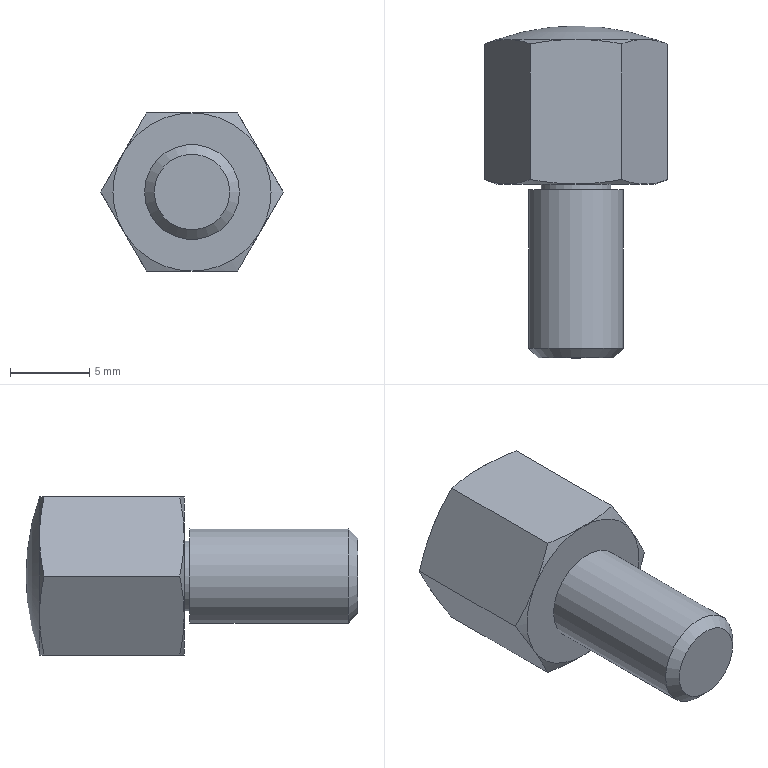Part | NX | features BREP 1 | 1 solid | 25 faces | box 11.547 x 21 x 10 mm | volume 1127 mm3 | cone 13 | plane 9 | cylinder 2 | sphere 1 | commonest cylinder face diameters 4.4 x1 6 x1
STEP:
#1=CARTESIAN_POINT('',(4.33,9.142,-2.5));
#2=VERTEX_POINT('',#1);
#3=CARTESIAN_POINT('',(4.33,9.142,2.5));
#4=VERTEX_POINT('',#3);
#5=CARTESIAN_POINT('',(0.,9.142,0.));
#6=DIRECTION('',(0.,-1.,0.));
#7=DIRECTION('',(1.,0.,0.));
#8=AXIS2_PLACEMENT_3D('',#5,#6,#7);
#9=CIRCLE('',#8,5.);
#10=EDGE_CURVE('',#2,#4,#9,.T.);
#11=ORIENTED_EDGE('',*,*,#10,.F.);
#12=CARTESIAN_POINT('',(0.,9.142,-5.));
#13=VERTEX_POINT('',#12);
#14=CARTESIAN_POINT('',(0.,9.142,0.));
#15=DIRECTION('',(0.,-1.,0.));
#16=DIRECTION('',(1.,0.,0.));
#17=AXIS2_PLACEMENT_3D('',#14,#15,#16);
#18=CIRCLE('',#17,5.);
#19=EDGE_CURVE('',#13,#2,#18,.T.);
#20=ORIENTED_EDGE('',*,*,#19,.F.);
#21=CARTESIAN_POINT('',(-4.33,9.142,-2.5));
#22=VERTEX_POINT('',#21);
#23=CARTESIAN_POINT('',(0.,9.142,0.));
#24=DIRECTION('',(0.,-1.,0.));
#25=DIRECTION('',(1.,0.,0.));
#26=AXIS2_PLACEMENT_3D('',#23,#24,#25);
#27=CIRCLE('',#26,5.);
#28=EDGE_CURVE('',#22,#13,#27,.T.);
#29=ORIENTED_EDGE('',*,*,#28,.F.);
#30=CARTESIAN_POINT('',(-4.33,9.142,2.5));
#31=VERTEX_POINT('',#30);
#32=CARTESIAN_POINT('',(0.,9.142,0.));
#33=DIRECTION('',(0.,-1.,0.));
#34=DIRECTION('',(1.,0.,0.));
#35=AXIS2_PLACEMENT_3D('',#32,#33,#34);
#36=CIRCLE('',#35,5.);
#37=EDGE_CURVE('',#31,#22,#36,.T.);
#38=ORIENTED_EDGE('',*,*,#37,.F.);
#39=CARTESIAN_POINT('',(0.,9.142,5.));
#40=VERTEX_POINT('',#39);
#41=CARTESIAN_POINT('',(0.,9.142,0.));
#42=DIRECTION('',(0.,-1.,0.));
#43=DIRECTION('',(1.,0.,0.));
#44=AXIS2_PLACEMENT_3D('',#41,#42,#43);
#45=CIRCLE('',#44,5.);
#46=EDGE_CURVE('',#40,#31,#45,.T.);
#47=ORIENTED_EDGE('',*,*,#46,.F.);
#48=CARTESIAN_POINT('',(0.,9.142,0.));
#49=DIRECTION('',(0.,-1.,0.));
#50=DIRECTION('',(1.,0.,0.));
#51=AXIS2_PLACEMENT_3D('',#48,#49,#50);
#52=CIRCLE('',#51,5.);
#53=EDGE_CURVE('',#4,#40,#52,.T.);
#54=ORIENTED_EDGE('',*,*,#53,.F.);
#55=EDGE_LOOP('',(#11,#20,#29,#38,#47,#54));
#56=FACE_BOUND('',#55,.T.);
#57=CARTESIAN_POINT('',(0.,-5.,0.));
#58=DIRECTION('',(0.,-1.,0.));
#59=DIRECTION('',(-1.,0.,0.));
#60=AXIS2_PLACEMENT_3D('',#57,#58,#59);
#61=SPHERICAL_SURFACE('',#60,15.);
#62=ADVANCED_FACE('',(#56),#61,.T.);
#63=CARTESIAN_POINT('',(2.2,0.,0.));
#64=VERTEX_POINT('',#63);
#65=CARTESIAN_POINT('',(0.,0.,0.));
#66=DIRECTION('',(0.,-1.,0.));
#67=DIRECTION('',(1.,0.,0.));
#68=AXIS2_PLACEMENT_3D('',#65,#66,#67);
#69=CIRCLE('',#68,2.2);
#70=EDGE_CURVE('',#64,#64,#69,.T.);
#71=ORIENTED_EDGE('',*,*,#70,.F.);
#72=EDGE_LOOP('',(#71));
#73=FACE_BOUND('',#72,.T.);
#74=CARTESIAN_POINT('',(4.33,0.,-2.5));
#75=VERTEX_POINT('',#74);
#76=CARTESIAN_POINT('',(4.33,0.,2.5));
#77=VERTEX_POINT('',#76);
#78=CARTESIAN_POINT('',(0.,0.,0.));
#79=DIRECTION('',(0.,-1.,0.));
#80=DIRECTION('',(1.,0.,0.));
#81=AXIS2_PLACEMENT_3D('',#78,#79,#80);
#82=CIRCLE('',#81,5.);
#83=EDGE_CURVE('',#75,#77,#82,.T.);
#84=ORIENTED_EDGE('',*,*,#83,.T.);
#85=CARTESIAN_POINT('',(0.,0.,5.));
#86=VERTEX_POINT('',#85);
#87=CARTESIAN_POINT('',(0.,0.,0.));
#88=DIRECTION('',(0.,-1.,0.));
#89=DIRECTION('',(1.,0.,0.));
#90=AXIS2_PLACEMENT_3D('',#87,#88,#89);
#91=CIRCLE('',#90,5.);
#92=EDGE_CURVE('',#77,#86,#91,.T.);
#93=ORIENTED_EDGE('',*,*,#92,.T.);
#94=CARTESIAN_POINT('',(-4.33,0.,2.5));
#95=VERTEX_POINT('',#94);
#96=CARTESIAN_POINT('',(0.,0.,0.));
#97=DIRECTION('',(0.,-1.,0.));
#98=DIRECTION('',(1.,0.,0.));
#99=AXIS2_PLACEMENT_3D('',#96,#97,#98);
#100=CIRCLE('',#99,5.);
#101=EDGE_CURVE('',#86,#95,#100,.T.);
#102=ORIENTED_EDGE('',*,*,#101,.T.);
#103=CARTESIAN_POINT('',(-4.33,0.,-2.5));
#104=VERTEX_POINT('',#103);
#105=CARTESIAN_POINT('',(0.,0.,0.));
#106=DIRECTION('',(0.,-1.,0.));
#107=DIRECTION('',(1.,0.,0.));
#108=AXIS2_PLACEMENT_3D('',#105,#106,#107);
#109=CIRCLE('',#108,5.);
#110=EDGE_CURVE('',#95,#104,#109,.T.);
#111=ORIENTED_EDGE('',*,*,#110,.T.);
#112=CARTESIAN_POINT('',(0.,0.,-5.));
#113=VERTEX_POINT('',#112);
#114=CARTESIAN_POINT('',(0.,0.,0.));
#115=DIRECTION('',(0.,-1.,0.));
#116=DIRECTION('',(1.,0.,0.));
#117=AXIS2_PLACEMENT_3D('',#114,#115,#116);
#118=CIRCLE('',#117,5.);
#119=EDGE_CURVE('',#104,#113,#118,.T.);
#120=ORIENTED_EDGE('',*,*,#119,.T.);
#121=CARTESIAN_POINT('',(0.,0.,0.));
#122=DIRECTION('',(0.,-1.,0.));
#123=DIRECTION('',(1.,0.,0.));
#124=AXIS2_PLACEMENT_3D('',#121,#122,#123);
#125=CIRCLE('',#124,5.);
#126=EDGE_CURVE('',#113,#75,#125,.T.);
#127=ORIENTED_EDGE('',*,*,#126,.T.);
#128=EDGE_LOOP('',(#84,#93,#102,#111,#120,#127));
#129=FACE_BOUND('',#128,.T.);
#130=CARTESIAN_POINT('',(3.6,0.,0.));
#131=DIRECTION('',(0.,-1.,0.));
#132=DIRECTION('',(0.,0.,-1.));
#133=AXIS2_PLACEMENT_3D('',#130,#131,#132);
#134=PLANE('',#133);
#135=ADVANCED_FACE('',(#73,#129),#134,.T.);
#136=CARTESIAN_POINT('',(2.2,-0.3667,0.));
#137=VERTEX_POINT('',#136);
#138=CARTESIAN_POINT('',(0.,-0.3667,0.));
#139=DIRECTION('',(0.,-1.,0.));
#140=DIRECTION('',(1.,0.,0.));
#141=AXIS2_PLACEMENT_3D('',#138,#139,#140);
#142=CIRCLE('',#141,2.2);
#143=EDGE_CURVE('',#137,#137,#142,.T.);
#144=ORIENTED_EDGE('',*,*,#143,.T.);
#145=EDGE_LOOP('',(#144));
#146=FACE_BOUND('',#145,.T.);
#147=CARTESIAN_POINT('',(3.,-0.3667,0.));
#148=VERTEX_POINT('',#147);
#149=CARTESIAN_POINT('',(0.,-0.3667,0.));
#150=DIRECTION('',(0.,-1.,0.));
#151=DIRECTION('',(1.,0.,0.));
#152=AXIS2_PLACEMENT_3D('',#149,#150,#151);
#153=CIRCLE('',#152,3.);
#154=EDGE_CURVE('',#148,#148,#153,.T.);
#155=ORIENTED_EDGE('',*,*,#154,.F.);
#156=EDGE_LOOP('',(#155));
#157=FACE_BOUND('',#156,.T.);
#158=CARTESIAN_POINT('',(2.6,-0.3667,0.));
#159=DIRECTION('',(0.,1.,0.));
#160=DIRECTION('',(-1.,0.,0.));
#161=AXIS2_PLACEMENT_3D('',#158,#159,#160);
#162=PLANE('',#161);
#163=ADVANCED_FACE('',(#146,#157),#162,.T.);
#164=CARTESIAN_POINT('',(2.386,-11.,0.));
#165=VERTEX_POINT('',#164);
#166=CARTESIAN_POINT('',(0.,-11.,0.));
#167=DIRECTION('',(0.,-1.,0.));
#168=DIRECTION('',(1.,0.,0.));
#169=AXIS2_PLACEMENT_3D('',#166,#167,#168);
#170=CIRCLE('',#169,2.386);
#171=EDGE_CURVE('',#165,#165,#170,.T.);
#172=ORIENTED_EDGE('',*,*,#171,.T.);
#173=EDGE_LOOP('',(#172));
#174=FACE_BOUND('',#173,.T.);
#175=CARTESIAN_POINT('',(1.193,-11.,0.));
#176=DIRECTION('',(0.,-1.,0.));
#177=DIRECTION('',(0.,0.,-1.));
#178=AXIS2_PLACEMENT_3D('',#175,#176,#177);
#179=PLANE('',#178);
#180=ADVANCED_FACE('',(#174),#179,.T.);
#181=CARTESIAN_POINT('',(-2.887,8.861,5.));
#182=VERTEX_POINT('',#181);
#183=CARTESIAN_POINT('',(0.,9.142,5.));
#184=CARTESIAN_POINT('',(-1.34,9.142,5.));
#185=CARTESIAN_POINT('',(-2.887,8.861,5.));
#186=(BOUNDED_CURVE()B_SPLINE_CURVE(2,(#183,#184,#185),.UNSPECIFIED.,.F.,.F.)B_SPLINE_CURVE_WITH_KNOTS((3,3),(0.,1.),.PIECEWISE_BEZIER_KNOTS.)CURVE()GEOMETRIC_REPRESENTATION_ITEM()RATIONAL_B_SPLINE_CURVE((1.,1.136,1.199))REPRESENTATION_ITEM(''));
#187=EDGE_CURVE('',#40,#182,#186,.T.);
#188=ORIENTED_EDGE('',*,*,#187,.F.);
#189=ORIENTED_EDGE('',*,*,#46,.T.);
#190=CARTESIAN_POINT('',(-2.887,8.861,5.));
#191=CARTESIAN_POINT('',(-3.66,9.142,3.66));
#192=CARTESIAN_POINT('',(-4.33,9.142,2.5));
#193=(BOUNDED_CURVE()B_SPLINE_CURVE(2,(#190,#191,#192),.UNSPECIFIED.,.F.,.F.)B_SPLINE_CURVE_WITH_KNOTS((3,3),(0.,1.),.PIECEWISE_BEZIER_KNOTS.)CURVE()GEOMETRIC_REPRESENTATION_ITEM()RATIONAL_B_SPLINE_CURVE((1.199,1.136,1.))REPRESENTATION_ITEM(''));
#194=EDGE_CURVE('',#182,#31,#193,.T.);
#195=ORIENTED_EDGE('',*,*,#194,.F.);
#196=EDGE_LOOP('',(#188,#189,#195));
#197=FACE_BOUND('',#196,.T.);
#198=CARTESIAN_POINT('',(0.,6.857,0.));
#199=DIRECTION('',(0.,-1.,0.));
#200=DIRECTION('',(-1.,0.,0.));
#201=AXIS2_PLACEMENT_3D('',#198,#199,#200);
#202=CONICAL_SURFACE('',#201,11.279,1.222);
#203=ADVANCED_FACE('',(#197),#202,.T.);
#204=CARTESIAN_POINT('',(2.887,8.861,5.));
#205=VERTEX_POINT('',#204);
#206=CARTESIAN_POINT('',(4.33,9.142,2.5));
#207=CARTESIAN_POINT('',(3.66,9.142,3.66));
#208=CARTESIAN_POINT('',(2.887,8.861,5.));
#209=(BOUNDED_CURVE()B_SPLINE_CURVE(2,(#206,#207,#208),.UNSPECIFIED.,.F.,.F.)B_SPLINE_CURVE_WITH_KNOTS((3,3),(0.,1.),.PIECEWISE_BEZIER_KNOTS.)CURVE()GEOMETRIC_REPRESENTATION_ITEM()RATIONAL_B_SPLINE_CURVE((1.,1.136,1.199))REPRESENTATION_ITEM(''));
#210=EDGE_CURVE('',#4,#205,#209,.T.);
#211=ORIENTED_EDGE('',*,*,#210,.F.);
#212=ORIENTED_EDGE('',*,*,#53,.T.);
#213=CARTESIAN_POINT('',(2.887,8.861,5.));
#214=CARTESIAN_POINT('',(1.34,9.142,5.));
#215=CARTESIAN_POINT('',(0.,9.142,5.));
#216=(BOUNDED_CURVE()B_SPLINE_CURVE(2,(#213,#214,#215),.UNSPECIFIED.,.F.,.F.)B_SPLINE_CURVE_WITH_KNOTS((3,3),(0.,1.),.PIECEWISE_BEZIER_KNOTS.)CURVE()GEOMETRIC_REPRESENTATION_ITEM()RATIONAL_B_SPLINE_CURVE((1.199,1.136,1.))REPRESENTATION_ITEM(''));
#217=EDGE_CURVE('',#205,#40,#216,.T.);
#218=ORIENTED_EDGE('',*,*,#217,.F.);
#219=EDGE_LOOP('',(#211,#212,#218));
#220=FACE_BOUND('',#219,.T.);
#221=CARTESIAN_POINT('',(0.,6.857,0.));
#222=DIRECTION('',(0.,-1.,0.));
#223=DIRECTION('',(-1.,0.,0.));
#224=AXIS2_PLACEMENT_3D('',#221,#222,#223);
#225=CONICAL_SURFACE('',#224,11.279,1.222);
#226=ADVANCED_FACE('',(#220),#225,.T.);
#227=CARTESIAN_POINT('',(2.887,8.861,-5.));
#228=VERTEX_POINT('',#227);
#229=CARTESIAN_POINT('',(2.887,8.861,-5.));
#230=CARTESIAN_POINT('',(3.66,9.142,-3.66));
#231=CARTESIAN_POINT('',(4.33,9.142,-2.5));
#232=(BOUNDED_CURVE()B_SPLINE_CURVE(2,(#229,#230,#231),.UNSPECIFIED.,.F.,.F.)B_SPLINE_CURVE_WITH_KNOTS((3,3),(0.,1.),.PIECEWISE_BEZIER_KNOTS.)CURVE()GEOMETRIC_REPRESENTATION_ITEM()RATIONAL_B_SPLINE_CURVE((1.199,1.136,1.))REPRESENTATION_ITEM(''));
#233=EDGE_CURVE('',#228,#2,#232,.T.);
#234=ORIENTED_EDGE('',*,*,#233,.F.);
#235=CARTESIAN_POINT('',(0.,9.142,-5.));
#236=CARTESIAN_POINT('',(1.34,9.142,-5.));
#237=CARTESIAN_POINT('',(2.887,8.861,-5.));
#238=(BOUNDED_CURVE()B_SPLINE_CURVE(2,(#235,#236,#237),.UNSPECIFIED.,.F.,.F.)B_SPLINE_CURVE_WITH_KNOTS((3,3),(0.,1.),.PIECEWISE_BEZIER_KNOTS.)CURVE()GEOMETRIC_REPRESENTATION_ITEM()RATIONAL_B_SPLINE_CURVE((1.,1.136,1.199))REPRESENTATION_ITEM(''));
#239=EDGE_CURVE('',#13,#228,#238,.T.);
#240=ORIENTED_EDGE('',*,*,#239,.F.);
#241=ORIENTED_EDGE('',*,*,#19,.T.);
#242=EDGE_LOOP('',(#234,#240,#241));
#243=FACE_BOUND('',#242,.T.);
#244=CARTESIAN_POINT('',(0.,6.857,0.));
#245=DIRECTION('',(0.,-1.,0.));
#246=DIRECTION('',(-1.,0.,0.));
#247=AXIS2_PLACEMENT_3D('',#244,#245,#246);
#248=CONICAL_SURFACE('',#247,11.279,1.222);
#249=ADVANCED_FACE('',(#243),#248,.T.);
#250=CARTESIAN_POINT('',(-2.887,8.861,-5.));
#251=VERTEX_POINT('',#250);
#252=CARTESIAN_POINT('',(-2.887,8.861,-5.));
#253=CARTESIAN_POINT('',(-1.34,9.142,-5.));
#254=CARTESIAN_POINT('',(0.,9.142,-5.));
#255=(BOUNDED_CURVE()B_SPLINE_CURVE(2,(#252,#253,#254),.UNSPECIFIED.,.F.,.F.)B_SPLINE_CURVE_WITH_KNOTS((3,3),(0.,1.),.PIECEWISE_BEZIER_KNOTS.)CURVE()GEOMETRIC_REPRESENTATION_ITEM()RATIONAL_B_SPLINE_CURVE((1.199,1.136,1.))REPRESENTATION_ITEM(''));
#256=EDGE_CURVE('',#251,#13,#255,.T.);
#257=ORIENTED_EDGE('',*,*,#256,.F.);
#258=CARTESIAN_POINT('',(-4.33,9.142,-2.5));
#259=CARTESIAN_POINT('',(-3.66,9.142,-3.66));
#260=CARTESIAN_POINT('',(-2.887,8.861,-5.));
#261=(BOUNDED_CURVE()B_SPLINE_CURVE(2,(#258,#259,#260),.UNSPECIFIED.,.F.,.F.)B_SPLINE_CURVE_WITH_KNOTS((3,3),(0.,1.),.PIECEWISE_BEZIER_KNOTS.)CURVE()GEOMETRIC_REPRESENTATION_ITEM()RATIONAL_B_SPLINE_CURVE((1.,1.136,1.199))REPRESENTATION_ITEM(''));
#262=EDGE_CURVE('',#22,#251,#261,.T.);
#263=ORIENTED_EDGE('',*,*,#262,.F.);
#264=ORIENTED_EDGE('',*,*,#28,.T.);
#265=EDGE_LOOP('',(#257,#263,#264));
#266=FACE_BOUND('',#265,.T.);
#267=CARTESIAN_POINT('',(0.,6.857,0.));
#268=DIRECTION('',(0.,-1.,0.));
#269=DIRECTION('',(-1.,0.,0.));
#270=AXIS2_PLACEMENT_3D('',#267,#268,#269);
#271=CONICAL_SURFACE('',#270,11.279,1.222);
#272=ADVANCED_FACE('',(#266),#271,.T.);
#273=CARTESIAN_POINT('',(-2.887,0.2815,5.));
#274=VERTEX_POINT('',#273);
#275=CARTESIAN_POINT('',(-4.33,0.,2.5));
#276=CARTESIAN_POINT('',(-3.66,0.,3.66));
#277=CARTESIAN_POINT('',(-2.887,0.2815,5.));
#278=(BOUNDED_CURVE()B_SPLINE_CURVE(2,(#275,#276,#277),.UNSPECIFIED.,.F.,.F.)B_SPLINE_CURVE_WITH_KNOTS((3,3),(0.,1.),.PIECEWISE_BEZIER_KNOTS.)CURVE()GEOMETRIC_REPRESENTATION_ITEM()RATIONAL_B_SPLINE_CURVE((1.,1.136,1.199))REPRESENTATION_ITEM(''));
#279=EDGE_CURVE('',#95,#274,#278,.T.);
#280=ORIENTED_EDGE('',*,*,#279,.F.);
#281=ORIENTED_EDGE('',*,*,#101,.F.);
#282=CARTESIAN_POINT('',(-2.887,0.2815,5.));
#283=CARTESIAN_POINT('',(-1.34,0.,5.));
#284=CARTESIAN_POINT('',(0.,0.,5.));
#285=(BOUNDED_CURVE()B_SPLINE_CURVE(2,(#282,#283,#284),.UNSPECIFIED.,.F.,.F.)B_SPLINE_CURVE_WITH_KNOTS((3,3),(0.,1.),.PIECEWISE_BEZIER_KNOTS.)CURVE()GEOMETRIC_REPRESENTATION_ITEM()RATIONAL_B_SPLINE_CURVE((1.199,1.136,1.))REPRESENTATION_ITEM(''));
#286=EDGE_CURVE('',#274,#86,#285,.T.);
#287=ORIENTED_EDGE('',*,*,#286,.F.);
#288=EDGE_LOOP('',(#280,#281,#287));
#289=FACE_BOUND('',#288,.T.);
#290=CARTESIAN_POINT('',(0.,2.286,0.));
#291=DIRECTION('',(0.,1.,0.));
#292=DIRECTION('',(-1.,0.,0.));
#293=AXIS2_PLACEMENT_3D('',#290,#291,#292);
#294=CONICAL_SURFACE('',#293,11.279,1.222);
#295=ADVANCED_FACE('',(#289),#294,.T.);
#296=CARTESIAN_POINT('',(-2.887,0.2815,-5.));
#297=VERTEX_POINT('',#296);
#298=CARTESIAN_POINT('',(0.,0.,-5.));
#299=CARTESIAN_POINT('',(-1.34,0.,-5.));
#300=CARTESIAN_POINT('',(-2.887,0.2815,-5.));
#301=(BOUNDED_CURVE()B_SPLINE_CURVE(2,(#298,#299,#300),.UNSPECIFIED.,.F.,.F.)B_SPLINE_CURVE_WITH_KNOTS((3,3),(0.,1.),.PIECEWISE_BEZIER_KNOTS.)CURVE()GEOMETRIC_REPRESENTATION_ITEM()RATIONAL_B_SPLINE_CURVE((1.,1.136,1.199))REPRESENTATION_ITEM(''));
#302=EDGE_CURVE('',#113,#297,#301,.T.);
#303=ORIENTED_EDGE('',*,*,#302,.F.);
#304=ORIENTED_EDGE('',*,*,#119,.F.);
#305=CARTESIAN_POINT('',(-2.887,0.2815,-5.));
#306=CARTESIAN_POINT('',(-3.66,0.,-3.66));
#307=CARTESIAN_POINT('',(-4.33,0.,-2.5));
#308=(BOUNDED_CURVE()B_SPLINE_CURVE(2,(#305,#306,#307),.UNSPECIFIED.,.F.,.F.)B_SPLINE_CURVE_WITH_KNOTS((3,3),(0.,1.),.PIECEWISE_BEZIER_KNOTS.)CURVE()GEOMETRIC_REPRESENTATION_ITEM()RATIONAL_B_SPLINE_CURVE((1.199,1.136,1.))REPRESENTATION_ITEM(''));
#309=EDGE_CURVE('',#297,#104,#308,.T.);
#310=ORIENTED_EDGE('',*,*,#309,.F.);
#311=EDGE_LOOP('',(#303,#304,#310));
#312=FACE_BOUND('',#311,.T.);
#313=CARTESIAN_POINT('',(0.,2.286,0.));
#314=DIRECTION('',(0.,1.,0.));
#315=DIRECTION('',(-1.,0.,0.));
#316=AXIS2_PLACEMENT_3D('',#313,#314,#315);
#317=CONICAL_SURFACE('',#316,11.279,1.222);
#318=ADVANCED_FACE('',(#312),#317,.T.);
#319=CARTESIAN_POINT('',(2.887,0.2815,-5.));
#320=VERTEX_POINT('',#319);
#321=CARTESIAN_POINT('',(2.887,0.2815,-5.));
#322=CARTESIAN_POINT('',(1.34,0.,-5.));
#323=CARTESIAN_POINT('',(0.,0.,-5.));
#324=(BOUNDED_CURVE()B_SPLINE_CURVE(2,(#321,#322,#323),.UNSPECIFIED.,.F.,.F.)B_SPLINE_CURVE_WITH_KNOTS((3,3),(0.,1.),.PIECEWISE_BEZIER_KNOTS.)CURVE()GEOMETRIC_REPRESENTATION_ITEM()RATIONAL_B_SPLINE_CURVE((1.199,1.136,1.))REPRESENTATION_ITEM(''));
#325=EDGE_CURVE('',#320,#113,#324,.T.);
#326=ORIENTED_EDGE('',*,*,#325,.F.);
#327=CARTESIAN_POINT('',(4.33,0.,-2.5));
#328=CARTESIAN_POINT('',(3.66,0.,-3.66));
#329=CARTESIAN_POINT('',(2.887,0.2815,-5.));
#330=(BOUNDED_CURVE()B_SPLINE_CURVE(2,(#327,#328,#329),.UNSPECIFIED.,.F.,.F.)B_SPLINE_CURVE_WITH_KNOTS((3,3),(0.,1.),.PIECEWISE_BEZIER_KNOTS.)CURVE()GEOMETRIC_REPRESENTATION_ITEM()RATIONAL_B_SPLINE_CURVE((1.,1.136,1.199))REPRESENTATION_ITEM(''));
#331=EDGE_CURVE('',#75,#320,#330,.T.);
#332=ORIENTED_EDGE('',*,*,#331,.F.);
#333=ORIENTED_EDGE('',*,*,#126,.F.);
#334=EDGE_LOOP('',(#326,#332,#333));
#335=FACE_BOUND('',#334,.T.);
#336=CARTESIAN_POINT('',(0.,2.286,0.));
#337=DIRECTION('',(0.,1.,0.));
#338=DIRECTION('',(-1.,0.,0.));
#339=AXIS2_PLACEMENT_3D('',#336,#337,#338);
#340=CONICAL_SURFACE('',#339,11.279,1.222);
#341=ADVANCED_FACE('',(#335),#340,.T.);
#342=CARTESIAN_POINT('',(2.887,0.2815,5.));
#343=VERTEX_POINT('',#342);
#344=CARTESIAN_POINT('',(2.887,0.2815,5.));
#345=CARTESIAN_POINT('',(3.66,0.,3.66));
#346=CARTESIAN_POINT('',(4.33,0.,2.5));
#347=(BOUNDED_CURVE()B_SPLINE_CURVE(2,(#344,#345,#346),.UNSPECIFIED.,.F.,.F.)B_SPLINE_CURVE_WITH_KNOTS((3,3),(0.,1.),.PIECEWISE_BEZIER_KNOTS.)CURVE()GEOMETRIC_REPRESENTATION_ITEM()RATIONAL_B_SPLINE_CURVE((1.199,1.136,1.))REPRESENTATION_ITEM(''));
#348=EDGE_CURVE('',#343,#77,#347,.T.);
#349=ORIENTED_EDGE('',*,*,#348,.F.);
#350=CARTESIAN_POINT('',(0.,0.,5.));
#351=CARTESIAN_POINT('',(1.34,0.,5.));
#352=CARTESIAN_POINT('',(2.887,0.2815,5.));
#353=(BOUNDED_CURVE()B_SPLINE_CURVE(2,(#350,#351,#352),.UNSPECIFIED.,.F.,.F.)B_SPLINE_CURVE_WITH_KNOTS((3,3),(0.,1.),.PIECEWISE_BEZIER_KNOTS.)CURVE()GEOMETRIC_REPRESENTATION_ITEM()RATIONAL_B_SPLINE_CURVE((1.,1.136,1.199))REPRESENTATION_ITEM(''));
#354=EDGE_CURVE('',#86,#343,#353,.T.);
#355=ORIENTED_EDGE('',*,*,#354,.F.);
#356=ORIENTED_EDGE('',*,*,#92,.F.);
#357=EDGE_LOOP('',(#349,#355,#356));
#358=FACE_BOUND('',#357,.T.);
#359=CARTESIAN_POINT('',(0.,2.286,0.));
#360=DIRECTION('',(0.,1.,0.));
#361=DIRECTION('',(-1.,0.,0.));
#362=AXIS2_PLACEMENT_3D('',#359,#360,#361);
#363=CONICAL_SURFACE('',#362,11.279,1.222);
#364=ADVANCED_FACE('',(#358),#363,.T.);
#365=ORIENTED_EDGE('',*,*,#331,.T.);
#366=CARTESIAN_POINT('',(2.887,15.,-5.));
#367=DIRECTION('',(0.,-1.,0.));
#368=VECTOR('',#367,1000.);
#369=LINE('',#366,#368);
#370=EDGE_CURVE('',#228,#320,#369,.T.);
#371=ORIENTED_EDGE('',*,*,#370,.F.);
#372=ORIENTED_EDGE('',*,*,#233,.T.);
#373=CARTESIAN_POINT('',(5.774,8.861,0.));
#374=VERTEX_POINT('',#373);
#375=CARTESIAN_POINT('',(4.33,9.142,-2.5));
#376=CARTESIAN_POINT('',(5.,9.142,-1.34));
#377=CARTESIAN_POINT('',(5.774,8.861,0.));
#378=(BOUNDED_CURVE()B_SPLINE_CURVE(2,(#375,#376,#377),.UNSPECIFIED.,.F.,.F.)B_SPLINE_CURVE_WITH_KNOTS((3,3),(0.,1.),.PIECEWISE_BEZIER_KNOTS.)CURVE()GEOMETRIC_REPRESENTATION_ITEM()RATIONAL_B_SPLINE_CURVE((1.,1.136,1.199))REPRESENTATION_ITEM(''));
#379=EDGE_CURVE('',#2,#374,#378,.T.);
#380=ORIENTED_EDGE('',*,*,#379,.T.);
#381=CARTESIAN_POINT('',(5.774,0.2815,0.));
#382=VERTEX_POINT('',#381);
#383=CARTESIAN_POINT('',(5.774,15.,0.));
#384=DIRECTION('',(0.,-1.,0.));
#385=VECTOR('',#384,1000.);
#386=LINE('',#383,#385);
#387=EDGE_CURVE('',#374,#382,#386,.T.);
#388=ORIENTED_EDGE('',*,*,#387,.T.);
#389=CARTESIAN_POINT('',(5.774,0.2815,0.));
#390=CARTESIAN_POINT('',(5.,0.,-1.34));
#391=CARTESIAN_POINT('',(4.33,0.,-2.5));
#392=(BOUNDED_CURVE()B_SPLINE_CURVE(2,(#389,#390,#391),.UNSPECIFIED.,.F.,.F.)B_SPLINE_CURVE_WITH_KNOTS((3,3),(0.,1.),.PIECEWISE_BEZIER_KNOTS.)CURVE()GEOMETRIC_REPRESENTATION_ITEM()RATIONAL_B_SPLINE_CURVE((1.199,1.136,1.))REPRESENTATION_ITEM(''));
#393=EDGE_CURVE('',#382,#75,#392,.T.);
#394=ORIENTED_EDGE('',*,*,#393,.T.);
#395=EDGE_LOOP('',(#365,#371,#372,#380,#388,#394));
#396=FACE_BOUND('',#395,.T.);
#397=CARTESIAN_POINT('',(5.774,15.,0.));
#398=DIRECTION('',(-0.866,0.,0.5));
#399=DIRECTION('',(0.5,0.,0.866));
#400=AXIS2_PLACEMENT_3D('',#397,#398,#399);
#401=PLANE('',#400);
#402=ADVANCED_FACE('',(#396),#401,.F.);
#403=CARTESIAN_POINT('',(4.33,0.,2.5));
#404=CARTESIAN_POINT('',(5.,0.,1.34));
#405=CARTESIAN_POINT('',(5.774,0.2815,0.));
#406=(BOUNDED_CURVE()B_SPLINE_CURVE(2,(#403,#404,#405),.UNSPECIFIED.,.F.,.F.)B_SPLINE_CURVE_WITH_KNOTS((3,3),(0.,1.),.PIECEWISE_BEZIER_KNOTS.)CURVE()GEOMETRIC_REPRESENTATION_ITEM()RATIONAL_B_SPLINE_CURVE((1.,1.136,1.199))REPRESENTATION_ITEM(''));
#407=EDGE_CURVE('',#77,#382,#406,.T.);
#408=ORIENTED_EDGE('',*,*,#407,.T.);
#409=ORIENTED_EDGE('',*,*,#387,.F.);
#410=CARTESIAN_POINT('',(5.774,8.861,0.));
#411=CARTESIAN_POINT('',(5.,9.142,1.34));
#412=CARTESIAN_POINT('',(4.33,9.142,2.5));
#413=(BOUNDED_CURVE()B_SPLINE_CURVE(2,(#410,#411,#412),.UNSPECIFIED.,.F.,.F.)B_SPLINE_CURVE_WITH_KNOTS((3,3),(0.,1.),.PIECEWISE_BEZIER_KNOTS.)CURVE()GEOMETRIC_REPRESENTATION_ITEM()RATIONAL_B_SPLINE_CURVE((1.199,1.136,1.))REPRESENTATION_ITEM(''));
#414=EDGE_CURVE('',#374,#4,#413,.T.);
#415=ORIENTED_EDGE('',*,*,#414,.T.);
#416=ORIENTED_EDGE('',*,*,#210,.T.);
#417=CARTESIAN_POINT('',(2.887,15.,5.));
#418=DIRECTION('',(0.,-1.,0.));
#419=VECTOR('',#418,1000.);
#420=LINE('',#417,#419);
#421=EDGE_CURVE('',#205,#343,#420,.T.);
#422=ORIENTED_EDGE('',*,*,#421,.T.);
#423=ORIENTED_EDGE('',*,*,#348,.T.);
#424=EDGE_LOOP('',(#408,#409,#415,#416,#422,#423));
#425=FACE_BOUND('',#424,.T.);
#426=CARTESIAN_POINT('',(2.887,15.,5.));
#427=DIRECTION('',(-0.866,0.,-0.5));
#428=DIRECTION('',(0.,-1.,0.));
#429=AXIS2_PLACEMENT_3D('',#426,#427,#428);
#430=PLANE('',#429);
#431=ADVANCED_FACE('',(#425),#430,.F.);
#432=ORIENTED_EDGE('',*,*,#354,.T.);
#433=ORIENTED_EDGE('',*,*,#421,.F.);
#434=ORIENTED_EDGE('',*,*,#217,.T.);
#435=ORIENTED_EDGE('',*,*,#187,.T.);
#436=CARTESIAN_POINT('',(-2.887,15.,5.));
#437=DIRECTION('',(0.,-1.,0.));
#438=VECTOR('',#437,1000.);
#439=LINE('',#436,#438);
#440=EDGE_CURVE('',#182,#274,#439,.T.);
#441=ORIENTED_EDGE('',*,*,#440,.T.);
#442=ORIENTED_EDGE('',*,*,#286,.T.);
#443=EDGE_LOOP('',(#432,#433,#434,#435,#441,#442));
#444=FACE_BOUND('',#443,.T.);
#445=CARTESIAN_POINT('',(-2.887,15.,5.));
#446=DIRECTION('',(0.,0.,-1.));
#447=DIRECTION('',(0.,1.,0.));
#448=AXIS2_PLACEMENT_3D('',#445,#446,#447);
#449=PLANE('',#448);
#450=ADVANCED_FACE('',(#444),#449,.F.);
#451=ORIENTED_EDGE('',*,*,#309,.T.);
#452=CARTESIAN_POINT('',(-5.774,0.2815,0.));
#453=VERTEX_POINT('',#452);
#454=CARTESIAN_POINT('',(-4.33,0.,-2.5));
#455=CARTESIAN_POINT('',(-5.,0.,-1.34));
#456=CARTESIAN_POINT('',(-5.774,0.2815,0.));
#457=(BOUNDED_CURVE()B_SPLINE_CURVE(2,(#454,#455,#456),.UNSPECIFIED.,.F.,.F.)B_SPLINE_CURVE_WITH_KNOTS((3,3),(0.,1.),.PIECEWISE_BEZIER_KNOTS.)CURVE()GEOMETRIC_REPRESENTATION_ITEM()RATIONAL_B_SPLINE_CURVE((1.,1.136,1.199))REPRESENTATION_ITEM(''));
#458=EDGE_CURVE('',#104,#453,#457,.T.);
#459=ORIENTED_EDGE('',*,*,#458,.T.);
#460=CARTESIAN_POINT('',(-5.774,8.861,0.));
#461=VERTEX_POINT('',#460);
#462=CARTESIAN_POINT('',(-5.774,15.,0.));
#463=DIRECTION('',(0.,-1.,0.));
#464=VECTOR('',#463,1000.);
#465=LINE('',#462,#464);
#466=EDGE_CURVE('',#461,#453,#465,.T.);
#467=ORIENTED_EDGE('',*,*,#466,.F.);
#468=CARTESIAN_POINT('',(-5.774,8.861,0.));
#469=CARTESIAN_POINT('',(-5.,9.142,-1.34));
#470=CARTESIAN_POINT('',(-4.33,9.142,-2.5));
#471=(BOUNDED_CURVE()B_SPLINE_CURVE(2,(#468,#469,#470),.UNSPECIFIED.,.F.,.F.)B_SPLINE_CURVE_WITH_KNOTS((3,3),(0.,1.),.PIECEWISE_BEZIER_KNOTS.)CURVE()GEOMETRIC_REPRESENTATION_ITEM()RATIONAL_B_SPLINE_CURVE((1.199,1.136,1.))REPRESENTATION_ITEM(''));
#472=EDGE_CURVE('',#461,#22,#471,.T.);
#473=ORIENTED_EDGE('',*,*,#472,.T.);
#474=ORIENTED_EDGE('',*,*,#262,.T.);
#475=CARTESIAN_POINT('',(-2.887,15.,-5.));
#476=DIRECTION('',(0.,-1.,0.));
#477=VECTOR('',#476,1000.);
#478=LINE('',#475,#477);
#479=EDGE_CURVE('',#251,#297,#478,.T.);
#480=ORIENTED_EDGE('',*,*,#479,.T.);
#481=EDGE_LOOP('',(#451,#459,#467,#473,#474,#480));
#482=FACE_BOUND('',#481,.T.);
#483=CARTESIAN_POINT('',(-2.887,15.,-5.));
#484=DIRECTION('',(0.866,0.,0.5));
#485=DIRECTION('',(0.,1.,0.));
#486=AXIS2_PLACEMENT_3D('',#483,#484,#485);
#487=PLANE('',#486);
#488=ADVANCED_FACE('',(#482),#487,.F.);
#489=CARTESIAN_POINT('',(-5.774,0.2815,0.));
#490=CARTESIAN_POINT('',(-5.,0.,1.34));
#491=CARTESIAN_POINT('',(-4.33,0.,2.5));
#492=(BOUNDED_CURVE()B_SPLINE_CURVE(2,(#489,#490,#491),.UNSPECIFIED.,.F.,.F.)B_SPLINE_CURVE_WITH_KNOTS((3,3),(0.,1.),.PIECEWISE_BEZIER_KNOTS.)CURVE()GEOMETRIC_REPRESENTATION_ITEM()RATIONAL_B_SPLINE_CURVE((1.199,1.136,1.))REPRESENTATION_ITEM(''));
#493=EDGE_CURVE('',#453,#95,#492,.T.);
#494=ORIENTED_EDGE('',*,*,#493,.T.);
#495=ORIENTED_EDGE('',*,*,#279,.T.);
#496=ORIENTED_EDGE('',*,*,#440,.F.);
#497=ORIENTED_EDGE('',*,*,#194,.T.);
#498=CARTESIAN_POINT('',(-4.33,9.142,2.5));
#499=CARTESIAN_POINT('',(-5.,9.142,1.34));
#500=CARTESIAN_POINT('',(-5.774,8.861,0.));
#501=(BOUNDED_CURVE()B_SPLINE_CURVE(2,(#498,#499,#500),.UNSPECIFIED.,.F.,.F.)B_SPLINE_CURVE_WITH_KNOTS((3,3),(0.,1.),.PIECEWISE_BEZIER_KNOTS.)CURVE()GEOMETRIC_REPRESENTATION_ITEM()RATIONAL_B_SPLINE_CURVE((1.,1.136,1.199))REPRESENTATION_ITEM(''));
#502=EDGE_CURVE('',#31,#461,#501,.T.);
#503=ORIENTED_EDGE('',*,*,#502,.T.);
#504=ORIENTED_EDGE('',*,*,#466,.T.);
#505=EDGE_LOOP('',(#494,#495,#496,#497,#503,#504));
#506=FACE_BOUND('',#505,.T.);
#507=CARTESIAN_POINT('',(-5.774,15.,0.));
#508=DIRECTION('',(0.866,0.,-0.5));
#509=DIRECTION('',(0.,1.,0.));
#510=AXIS2_PLACEMENT_3D('',#507,#508,#509);
#511=PLANE('',#510);
#512=ADVANCED_FACE('',(#506),#511,.F.);
#513=ORIENTED_EDGE('',*,*,#325,.T.);
#514=ORIENTED_EDGE('',*,*,#302,.T.);
#515=ORIENTED_EDGE('',*,*,#479,.F.);
#516=ORIENTED_EDGE('',*,*,#256,.T.);
#517=ORIENTED_EDGE('',*,*,#239,.T.);
#518=ORIENTED_EDGE('',*,*,#370,.T.);
#519=EDGE_LOOP('',(#513,#514,#515,#516,#517,#518));
#520=FACE_BOUND('',#519,.T.);
#521=CARTESIAN_POINT('',(2.887,15.,-5.));
#522=DIRECTION('',(0.,0.,1.));
#523=DIRECTION('',(1.,0.,0.));
#524=AXIS2_PLACEMENT_3D('',#521,#522,#523);
#525=PLANE('',#524);
#526=ADVANCED_FACE('',(#520),#525,.F.);
#527=ORIENTED_EDGE('',*,*,#407,.F.);
#528=ORIENTED_EDGE('',*,*,#83,.F.);
#529=ORIENTED_EDGE('',*,*,#393,.F.);
#530=EDGE_LOOP('',(#527,#528,#529));
#531=FACE_BOUND('',#530,.T.);
#532=CARTESIAN_POINT('',(0.,2.286,0.));
#533=DIRECTION('',(0.,1.,0.));
#534=DIRECTION('',(-1.,0.,0.));
#535=AXIS2_PLACEMENT_3D('',#532,#533,#534);
#536=CONICAL_SURFACE('',#535,11.279,1.222);
#537=ADVANCED_FACE('',(#531),#536,.T.);
#538=ORIENTED_EDGE('',*,*,#110,.F.);
#539=ORIENTED_EDGE('',*,*,#493,.F.);
#540=ORIENTED_EDGE('',*,*,#458,.F.);
#541=EDGE_LOOP('',(#538,#539,#540));
#542=FACE_BOUND('',#541,.T.);
#543=CARTESIAN_POINT('',(0.,2.286,0.));
#544=DIRECTION('',(0.,1.,0.));
#545=DIRECTION('',(-1.,0.,0.));
#546=AXIS2_PLACEMENT_3D('',#543,#544,#545);
#547=CONICAL_SURFACE('',#546,11.279,1.222);
#548=ADVANCED_FACE('',(#542),#547,.T.);
#549=ORIENTED_EDGE('',*,*,#10,.T.);
#550=ORIENTED_EDGE('',*,*,#414,.F.);
#551=ORIENTED_EDGE('',*,*,#379,.F.);
#552=EDGE_LOOP('',(#549,#550,#551));
#553=FACE_BOUND('',#552,.T.);
#554=CARTESIAN_POINT('',(0.,6.857,0.));
#555=DIRECTION('',(0.,-1.,0.));
#556=DIRECTION('',(-1.,0.,0.));
#557=AXIS2_PLACEMENT_3D('',#554,#555,#556);
#558=CONICAL_SURFACE('',#557,11.279,1.222);
#559=ADVANCED_FACE('',(#553),#558,.T.);
#560=ORIENTED_EDGE('',*,*,#502,.F.);
#561=ORIENTED_EDGE('',*,*,#37,.T.);
#562=ORIENTED_EDGE('',*,*,#472,.F.);
#563=EDGE_LOOP('',(#560,#561,#562));
#564=FACE_BOUND('',#563,.T.);
#565=CARTESIAN_POINT('',(0.,6.857,0.));
#566=DIRECTION('',(0.,-1.,0.));
#567=DIRECTION('',(-1.,0.,0.));
#568=AXIS2_PLACEMENT_3D('',#565,#566,#567);
#569=CONICAL_SURFACE('',#568,11.279,1.222);
#570=ADVANCED_FACE('',(#564),#569,.T.);
#571=ORIENTED_EDGE('',*,*,#171,.F.);
#572=EDGE_LOOP('',(#571));
#573=FACE_BOUND('',#572,.T.);
#574=CARTESIAN_POINT('',(3.,-10.386,0.));
#575=VERTEX_POINT('',#574);
#576=CARTESIAN_POINT('',(0.,-10.386,0.));
#577=DIRECTION('',(0.,-1.,0.));
#578=DIRECTION('',(1.,0.,0.));
#579=AXIS2_PLACEMENT_3D('',#576,#577,#578);
#580=CIRCLE('',#579,3.);
#581=EDGE_CURVE('',#575,#575,#580,.T.);
#582=ORIENTED_EDGE('',*,*,#581,.T.);
#583=EDGE_LOOP('',(#582));
#584=FACE_BOUND('',#583,.T.);
#585=CARTESIAN_POINT('',(0.,-10.693,0.));
#586=DIRECTION('',(0.,1.,0.));
#587=DIRECTION('',(-1.,0.,0.));
#588=AXIS2_PLACEMENT_3D('',#585,#586,#587);
#589=CONICAL_SURFACE('',#588,2.693,0.7854);
#590=ADVANCED_FACE('',(#573,#584),#589,.T.);
#591=ORIENTED_EDGE('',*,*,#581,.F.);
#592=EDGE_LOOP('',(#591));
#593=FACE_BOUND('',#592,.T.);
#594=ORIENTED_EDGE('',*,*,#154,.T.);
#595=EDGE_LOOP('',(#594));
#596=FACE_BOUND('',#595,.T.);
#597=CARTESIAN_POINT('',(0.,-5.377,0.));
#598=DIRECTION('',(0.,1.,0.));
#599=DIRECTION('',(-1.,0.,0.));
#600=AXIS2_PLACEMENT_3D('',#597,#598,#599);
#601=CYLINDRICAL_SURFACE('',#600,3.);
#602=ADVANCED_FACE('',(#593,#596),#601,.T.);
#603=ORIENTED_EDGE('',*,*,#143,.F.);
#604=EDGE_LOOP('',(#603));
#605=FACE_BOUND('',#604,.T.);
#606=ORIENTED_EDGE('',*,*,#70,.T.);
#607=EDGE_LOOP('',(#606));
#608=FACE_BOUND('',#607,.T.);
#609=CARTESIAN_POINT('',(0.,-0.1833,0.));
#610=DIRECTION('',(0.,1.,0.));
#611=DIRECTION('',(-1.,0.,0.));
#612=AXIS2_PLACEMENT_3D('',#609,#610,#611);
#613=CYLINDRICAL_SURFACE('',#612,2.2);
#614=ADVANCED_FACE('',(#605,#608),#613,.T.);
#615=CLOSED_SHELL('',(#62,#135,#163,#180,#203,#226,#249,#272,#295,#318,#341,#364,#402,#431,#450,#488,#512,#526,#537,#548,#559,#570,#590,#602,#614));
#616=MANIFOLD_SOLID_BREP('',#615);
#617=(LENGTH_UNIT()NAMED_UNIT(*)SI_UNIT(.MILLI.,.METRE.));
#618=UNCERTAINTY_MEASURE_WITH_UNIT(LENGTH_MEASURE(0.00001),#617,'','');
#619=(NAMED_UNIT(*)PLANE_ANGLE_UNIT()SI_UNIT($,.RADIAN.));
#620=(NAMED_UNIT(*)SI_UNIT($,.STERADIAN.)SOLID_ANGLE_UNIT());
#621=(GEOMETRIC_REPRESENTATION_CONTEXT(3)GLOBAL_UNCERTAINTY_ASSIGNED_CONTEXT((#618))GLOBAL_UNIT_ASSIGNED_CONTEXT((#617,#619,#620))REPRESENTATION_CONTEXT('',''));
#622=ADVANCED_BREP_SHAPE_REPRESENTATION('',(#616),#621);